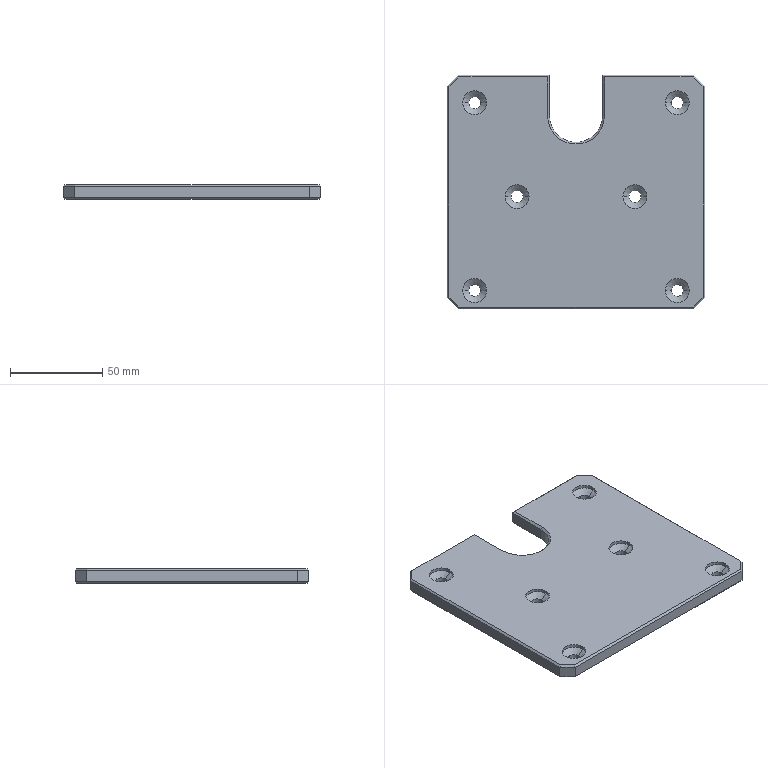Part | Creo | 1 solid | 74 faces | box 140 x 127 x 8 mm | volume 129995 mm3 | plane 35 | cylinder 25 | cone 14 | commonest cylinder face diameters 6.6 x12 13 x12 29 x1